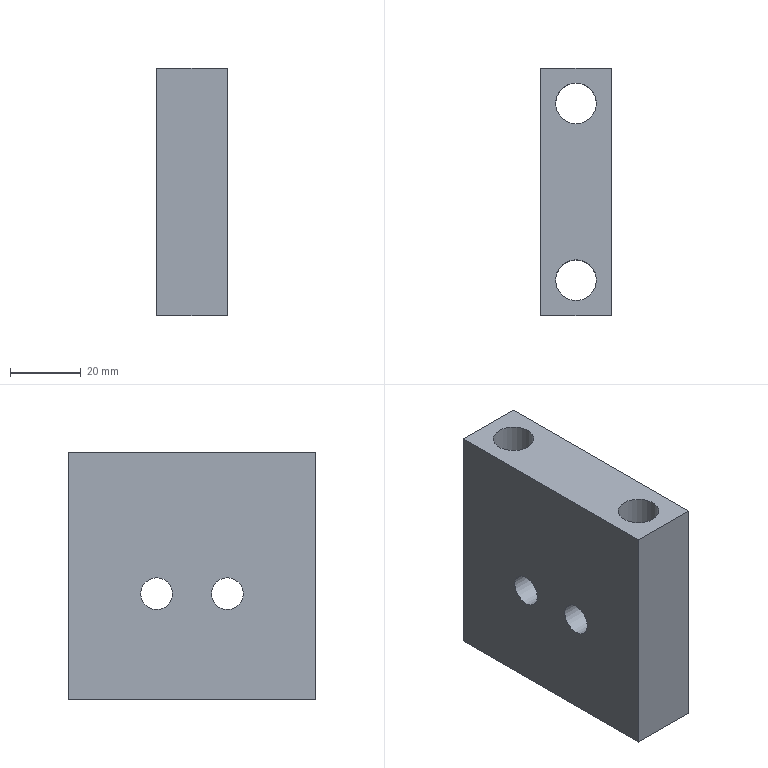Part | NX | features solid 2 | 1 solid | 18 faces | box 20 x 70 x 70 mm | volume 74709 mm3 | plane 10 | cylinder 8 | commonest cylinder face diameters 9 x2 11.5 x2 14 x2 16.5 x2
STEP:
#1=CARTESIAN_POINT('',(-199.,160.,174.5));
#2=VERTEX_POINT('',#1);
#3=CARTESIAN_POINT('',(-199.,160.,170.));
#4=DIRECTION('',(1.,0.,0.));
#5=DIRECTION('',(0.,0.,1.));
#6=AXIS2_PLACEMENT_3D('',#3,#4,#5);
#7=CIRCLE('',#6,4.5);
#8=EDGE_CURVE('',#2,#2,#7,.T.);
#9=ORIENTED_EDGE('',*,*,#8,.T.);
#10=EDGE_LOOP('',(#9));
#11=FACE_BOUND('',#10,.T.);
#12=CARTESIAN_POINT('',(-199.,180.,174.5));
#13=VERTEX_POINT('',#12);
#14=CARTESIAN_POINT('',(-199.,180.,170.));
#15=DIRECTION('',(1.,0.,0.));
#16=DIRECTION('',(0.,0.,1.));
#17=AXIS2_PLACEMENT_3D('',#14,#15,#16);
#18=CIRCLE('',#17,4.5);
#19=EDGE_CURVE('',#13,#13,#18,.T.);
#20=ORIENTED_EDGE('',*,*,#19,.T.);
#21=EDGE_LOOP('',(#20));
#22=FACE_BOUND('',#21,.T.);
#23=CARTESIAN_POINT('',(-199.,205.,210.));
#24=VERTEX_POINT('',#23);
#25=CARTESIAN_POINT('',(-199.,205.,140.));
#26=VERTEX_POINT('',#25);
#27=CARTESIAN_POINT('',(-199.,205.,197.5));
#28=DIRECTION('',(0.,0.,1.));
#29=VECTOR('',#28,1000.);
#30=LINE('',#27,#29);
#31=EDGE_CURVE('',#24,#26,#30,.F.);
#32=ORIENTED_EDGE('',*,*,#31,.T.);
#33=CARTESIAN_POINT('',(-199.,135.,140.));
#34=VERTEX_POINT('',#33);
#35=CARTESIAN_POINT('',(-199.,200.,140.));
#36=DIRECTION('',(0.,-1.,0.));
#37=VECTOR('',#36,1000.);
#38=LINE('',#35,#37);
#39=EDGE_CURVE('',#26,#34,#38,.T.);
#40=ORIENTED_EDGE('',*,*,#39,.T.);
#41=CARTESIAN_POINT('',(-199.,135.,210.));
#42=VERTEX_POINT('',#41);
#43=CARTESIAN_POINT('',(-199.,135.,197.5));
#44=DIRECTION('',(0.,0.,-1.));
#45=VECTOR('',#44,1000.);
#46=LINE('',#43,#45);
#47=EDGE_CURVE('',#42,#34,#46,.T.);
#48=ORIENTED_EDGE('',*,*,#47,.F.);
#49=CARTESIAN_POINT('',(-199.,200.,210.));
#50=DIRECTION('',(0.,-1.,0.));
#51=VECTOR('',#50,1000.);
#52=LINE('',#49,#51);
#53=EDGE_CURVE('',#24,#42,#52,.T.);
#54=ORIENTED_EDGE('',*,*,#53,.F.);
#55=EDGE_LOOP('',(#32,#40,#48,#54));
#56=FACE_BOUND('',#55,.T.);
#57=CARTESIAN_POINT('',(-199.,200.,197.5));
#58=DIRECTION('',(-1.,0.,0.));
#59=DIRECTION('',(0.,-1.,0.));
#60=AXIS2_PLACEMENT_3D('',#57,#58,#59);
#61=PLANE('',#60);
#62=ADVANCED_FACE('',(#11,#22,#56),#61,.T.);
#63=ORIENTED_EDGE('',*,*,#47,.T.);
#64=CARTESIAN_POINT('',(-179.,135.,140.));
#65=VERTEX_POINT('',#64);
#66=CARTESIAN_POINT('',(-199.,135.,140.));
#67=DIRECTION('',(1.,0.,0.));
#68=VECTOR('',#67,1000.);
#69=LINE('',#66,#68);
#70=EDGE_CURVE('',#34,#65,#69,.T.);
#71=ORIENTED_EDGE('',*,*,#70,.T.);
#72=CARTESIAN_POINT('',(-179.,135.,210.));
#73=VERTEX_POINT('',#72);
#74=CARTESIAN_POINT('',(-179.,135.,197.5));
#75=DIRECTION('',(0.,0.,1.));
#76=VECTOR('',#75,1000.);
#77=LINE('',#74,#76);
#78=EDGE_CURVE('',#73,#65,#77,.F.);
#79=ORIENTED_EDGE('',*,*,#78,.F.);
#80=CARTESIAN_POINT('',(-199.,135.,210.));
#81=DIRECTION('',(1.,0.,0.));
#82=VECTOR('',#81,1000.);
#83=LINE('',#80,#82);
#84=EDGE_CURVE('',#42,#73,#83,.T.);
#85=ORIENTED_EDGE('',*,*,#84,.F.);
#86=EDGE_LOOP('',(#63,#71,#79,#85));
#87=FACE_BOUND('',#86,.T.);
#88=CARTESIAN_POINT('',(-199.,135.,197.5));
#89=DIRECTION('',(0.,-1.,0.));
#90=DIRECTION('',(1.,0.,0.));
#91=AXIS2_PLACEMENT_3D('',#88,#89,#90);
#92=PLANE('',#91);
#93=ADVANCED_FACE('',(#87),#92,.T.);
#94=CARTESIAN_POINT('',(-179.,160.,177.));
#95=VERTEX_POINT('',#94);
#96=CARTESIAN_POINT('',(-179.,160.,170.));
#97=DIRECTION('',(1.,0.,0.));
#98=DIRECTION('',(0.,0.,1.));
#99=AXIS2_PLACEMENT_3D('',#96,#97,#98);
#100=CIRCLE('',#99,7.);
#101=EDGE_CURVE('',#95,#95,#100,.T.);
#102=ORIENTED_EDGE('',*,*,#101,.F.);
#103=EDGE_LOOP('',(#102));
#104=FACE_BOUND('',#103,.T.);
#105=CARTESIAN_POINT('',(-179.,180.,177.));
#106=VERTEX_POINT('',#105);
#107=CARTESIAN_POINT('',(-179.,180.,170.));
#108=DIRECTION('',(1.,0.,0.));
#109=DIRECTION('',(0.,0.,1.));
#110=AXIS2_PLACEMENT_3D('',#107,#108,#109);
#111=CIRCLE('',#110,7.);
#112=EDGE_CURVE('',#106,#106,#111,.T.);
#113=ORIENTED_EDGE('',*,*,#112,.F.);
#114=EDGE_LOOP('',(#113));
#115=FACE_BOUND('',#114,.T.);
#116=ORIENTED_EDGE('',*,*,#78,.T.);
#117=CARTESIAN_POINT('',(-179.,205.,140.));
#118=VERTEX_POINT('',#117);
#119=CARTESIAN_POINT('',(-179.,200.,140.));
#120=DIRECTION('',(0.,1.,0.));
#121=VECTOR('',#120,1000.);
#122=LINE('',#119,#121);
#123=EDGE_CURVE('',#118,#65,#122,.F.);
#124=ORIENTED_EDGE('',*,*,#123,.F.);
#125=CARTESIAN_POINT('',(-179.,205.,210.));
#126=VERTEX_POINT('',#125);
#127=CARTESIAN_POINT('',(-179.,205.,197.5));
#128=DIRECTION('',(0.,0.,-1.));
#129=VECTOR('',#128,1000.);
#130=LINE('',#127,#129);
#131=EDGE_CURVE('',#126,#118,#130,.T.);
#132=ORIENTED_EDGE('',*,*,#131,.F.);
#133=CARTESIAN_POINT('',(-179.,200.,210.));
#134=DIRECTION('',(0.,1.,0.));
#135=VECTOR('',#134,1000.);
#136=LINE('',#133,#135);
#137=EDGE_CURVE('',#126,#73,#136,.F.);
#138=ORIENTED_EDGE('',*,*,#137,.T.);
#139=EDGE_LOOP('',(#116,#124,#132,#138));
#140=FACE_BOUND('',#139,.T.);
#141=CARTESIAN_POINT('',(-179.,200.,197.5));
#142=DIRECTION('',(-1.,0.,0.));
#143=DIRECTION('',(0.,-1.,0.));
#144=AXIS2_PLACEMENT_3D('',#141,#142,#143);
#145=PLANE('',#144);
#146=ADVANCED_FACE('',(#104,#115,#140),#145,.F.);
#147=CARTESIAN_POINT('',(-199.,205.,210.));
#148=DIRECTION('',(-1.,0.,0.));
#149=VECTOR('',#148,1000.);
#150=LINE('',#147,#149);
#151=EDGE_CURVE('',#24,#126,#150,.F.);
#152=ORIENTED_EDGE('',*,*,#151,.T.);
#153=ORIENTED_EDGE('',*,*,#131,.T.);
#154=CARTESIAN_POINT('',(-199.,205.,140.));
#155=DIRECTION('',(-1.,0.,0.));
#156=VECTOR('',#155,1000.);
#157=LINE('',#154,#156);
#158=EDGE_CURVE('',#26,#118,#157,.F.);
#159=ORIENTED_EDGE('',*,*,#158,.F.);
#160=ORIENTED_EDGE('',*,*,#31,.F.);
#161=EDGE_LOOP('',(#152,#153,#159,#160));
#162=FACE_BOUND('',#161,.T.);
#163=CARTESIAN_POINT('',(-199.,205.,197.5));
#164=DIRECTION('',(0.,-1.,0.));
#165=DIRECTION('',(1.,0.,0.));
#166=AXIS2_PLACEMENT_3D('',#163,#164,#165);
#167=PLANE('',#166);
#168=ADVANCED_FACE('',(#162),#167,.F.);
#169=CARTESIAN_POINT('',(-189.,186.75,140.));
#170=VERTEX_POINT('',#169);
#171=CARTESIAN_POINT('',(-189.,195.,140.));
#172=DIRECTION('',(0.,0.,-1.));
#173=DIRECTION('',(0.,-1.,0.));
#174=AXIS2_PLACEMENT_3D('',#171,#172,#173);
#175=CIRCLE('',#174,8.25);
#176=EDGE_CURVE('',#170,#170,#175,.T.);
#177=ORIENTED_EDGE('',*,*,#176,.F.);
#178=EDGE_LOOP('',(#177));
#179=FACE_BOUND('',#178,.T.);
#180=CARTESIAN_POINT('',(-189.,136.75,140.));
#181=VERTEX_POINT('',#180);
#182=CARTESIAN_POINT('',(-189.,145.,140.));
#183=DIRECTION('',(0.,0.,-1.));
#184=DIRECTION('',(0.,-1.,0.));
#185=AXIS2_PLACEMENT_3D('',#182,#183,#184);
#186=CIRCLE('',#185,8.25);
#187=EDGE_CURVE('',#181,#181,#186,.T.);
#188=ORIENTED_EDGE('',*,*,#187,.F.);
#189=EDGE_LOOP('',(#188));
#190=FACE_BOUND('',#189,.T.);
#191=ORIENTED_EDGE('',*,*,#123,.T.);
#192=ORIENTED_EDGE('',*,*,#70,.F.);
#193=ORIENTED_EDGE('',*,*,#39,.F.);
#194=ORIENTED_EDGE('',*,*,#158,.T.);
#195=EDGE_LOOP('',(#191,#192,#193,#194));
#196=FACE_BOUND('',#195,.T.);
#197=CARTESIAN_POINT('',(-199.,200.,140.));
#198=DIRECTION('',(0.,0.,-1.));
#199=DIRECTION('',(0.,1.,0.));
#200=AXIS2_PLACEMENT_3D('',#197,#198,#199);
#201=PLANE('',#200);
#202=ADVANCED_FACE('',(#179,#190,#196),#201,.T.);
#203=CARTESIAN_POINT('',(-189.,200.75,210.));
#204=VERTEX_POINT('',#203);
#205=CARTESIAN_POINT('',(-189.,195.,210.));
#206=DIRECTION('',(0.,0.,1.));
#207=DIRECTION('',(0.,1.,0.));
#208=AXIS2_PLACEMENT_3D('',#205,#206,#207);
#209=CIRCLE('',#208,5.75);
#210=EDGE_CURVE('',#204,#204,#209,.T.);
#211=ORIENTED_EDGE('',*,*,#210,.F.);
#212=EDGE_LOOP('',(#211));
#213=FACE_BOUND('',#212,.T.);
#214=CARTESIAN_POINT('',(-189.,150.75,210.));
#215=VERTEX_POINT('',#214);
#216=CARTESIAN_POINT('',(-189.,145.,210.));
#217=DIRECTION('',(0.,0.,1.));
#218=DIRECTION('',(0.,1.,0.));
#219=AXIS2_PLACEMENT_3D('',#216,#217,#218);
#220=CIRCLE('',#219,5.75);
#221=EDGE_CURVE('',#215,#215,#220,.T.);
#222=ORIENTED_EDGE('',*,*,#221,.F.);
#223=EDGE_LOOP('',(#222));
#224=FACE_BOUND('',#223,.T.);
#225=ORIENTED_EDGE('',*,*,#137,.F.);
#226=ORIENTED_EDGE('',*,*,#151,.F.);
#227=ORIENTED_EDGE('',*,*,#53,.T.);
#228=ORIENTED_EDGE('',*,*,#84,.T.);
#229=EDGE_LOOP('',(#225,#226,#227,#228));
#230=FACE_BOUND('',#229,.T.);
#231=CARTESIAN_POINT('',(-199.,200.,210.));
#232=DIRECTION('',(0.,0.,-1.));
#233=DIRECTION('',(0.,1.,0.));
#234=AXIS2_PLACEMENT_3D('',#231,#232,#233);
#235=PLANE('',#234);
#236=ADVANCED_FACE('',(#213,#224,#230),#235,.F.);
#237=ORIENTED_EDGE('',*,*,#19,.F.);
#238=EDGE_LOOP('',(#237));
#239=FACE_BOUND('',#238,.T.);
#240=CARTESIAN_POINT('',(-189.,180.,174.5));
#241=VERTEX_POINT('',#240);
#242=CARTESIAN_POINT('',(-189.,180.,170.));
#243=DIRECTION('',(1.,0.,0.));
#244=DIRECTION('',(0.,0.,1.));
#245=AXIS2_PLACEMENT_3D('',#242,#243,#244);
#246=CIRCLE('',#245,4.5);
#247=EDGE_CURVE('',#241,#241,#246,.T.);
#248=ORIENTED_EDGE('',*,*,#247,.T.);
#249=EDGE_LOOP('',(#248));
#250=FACE_BOUND('',#249,.T.);
#251=CARTESIAN_POINT('',(-229.,180.,170.));
#252=DIRECTION('',(-1.,0.,0.));
#253=DIRECTION('',(0.,0.,1.));
#254=AXIS2_PLACEMENT_3D('',#251,#252,#253);
#255=CYLINDRICAL_SURFACE('',#254,4.5);
#256=ADVANCED_FACE('',(#239,#250),#255,.F.);
#257=ORIENTED_EDGE('',*,*,#247,.F.);
#258=EDGE_LOOP('',(#257));
#259=FACE_BOUND('',#258,.T.);
#260=CARTESIAN_POINT('',(-189.,180.,177.));
#261=VERTEX_POINT('',#260);
#262=CARTESIAN_POINT('',(-189.,180.,170.));
#263=DIRECTION('',(1.,0.,0.));
#264=DIRECTION('',(0.,0.,1.));
#265=AXIS2_PLACEMENT_3D('',#262,#263,#264);
#266=CIRCLE('',#265,7.);
#267=EDGE_CURVE('',#261,#261,#266,.T.);
#268=ORIENTED_EDGE('',*,*,#267,.T.);
#269=EDGE_LOOP('',(#268));
#270=FACE_BOUND('',#269,.T.);
#271=CARTESIAN_POINT('',(-189.,180.,170.));
#272=DIRECTION('',(-1.,0.,0.));
#273=DIRECTION('',(0.,0.,1.));
#274=AXIS2_PLACEMENT_3D('',#271,#272,#273);
#275=PLANE('',#274);
#276=ADVANCED_FACE('',(#259,#270),#275,.F.);
#277=ORIENTED_EDGE('',*,*,#267,.F.);
#278=EDGE_LOOP('',(#277));
#279=FACE_BOUND('',#278,.T.);
#280=ORIENTED_EDGE('',*,*,#112,.T.);
#281=EDGE_LOOP('',(#280));
#282=FACE_BOUND('',#281,.T.);
#283=CARTESIAN_POINT('',(-179.,180.,170.));
#284=DIRECTION('',(-1.,0.,0.));
#285=DIRECTION('',(0.,0.,1.));
#286=AXIS2_PLACEMENT_3D('',#283,#284,#285);
#287=CYLINDRICAL_SURFACE('',#286,7.);
#288=ADVANCED_FACE('',(#279,#282),#287,.F.);
#289=ORIENTED_EDGE('',*,*,#8,.F.);
#290=EDGE_LOOP('',(#289));
#291=FACE_BOUND('',#290,.T.);
#292=CARTESIAN_POINT('',(-189.,160.,174.5));
#293=VERTEX_POINT('',#292);
#294=CARTESIAN_POINT('',(-189.,160.,170.));
#295=DIRECTION('',(1.,0.,0.));
#296=DIRECTION('',(0.,0.,1.));
#297=AXIS2_PLACEMENT_3D('',#294,#295,#296);
#298=CIRCLE('',#297,4.5);
#299=EDGE_CURVE('',#293,#293,#298,.T.);
#300=ORIENTED_EDGE('',*,*,#299,.T.);
#301=EDGE_LOOP('',(#300));
#302=FACE_BOUND('',#301,.T.);
#303=CARTESIAN_POINT('',(-229.,160.,170.));
#304=DIRECTION('',(-1.,0.,0.));
#305=DIRECTION('',(0.,0.,1.));
#306=AXIS2_PLACEMENT_3D('',#303,#304,#305);
#307=CYLINDRICAL_SURFACE('',#306,4.5);
#308=ADVANCED_FACE('',(#291,#302),#307,.F.);
#309=ORIENTED_EDGE('',*,*,#299,.F.);
#310=EDGE_LOOP('',(#309));
#311=FACE_BOUND('',#310,.T.);
#312=CARTESIAN_POINT('',(-189.,160.,177.));
#313=VERTEX_POINT('',#312);
#314=CARTESIAN_POINT('',(-189.,160.,170.));
#315=DIRECTION('',(1.,0.,0.));
#316=DIRECTION('',(0.,0.,1.));
#317=AXIS2_PLACEMENT_3D('',#314,#315,#316);
#318=CIRCLE('',#317,7.);
#319=EDGE_CURVE('',#313,#313,#318,.T.);
#320=ORIENTED_EDGE('',*,*,#319,.T.);
#321=EDGE_LOOP('',(#320));
#322=FACE_BOUND('',#321,.T.);
#323=CARTESIAN_POINT('',(-189.,160.,170.));
#324=DIRECTION('',(-1.,0.,0.));
#325=DIRECTION('',(0.,0.,1.));
#326=AXIS2_PLACEMENT_3D('',#323,#324,#325);
#327=PLANE('',#326);
#328=ADVANCED_FACE('',(#311,#322),#327,.F.);
#329=ORIENTED_EDGE('',*,*,#319,.F.);
#330=EDGE_LOOP('',(#329));
#331=FACE_BOUND('',#330,.T.);
#332=ORIENTED_EDGE('',*,*,#101,.T.);
#333=EDGE_LOOP('',(#332));
#334=FACE_BOUND('',#333,.T.);
#335=CARTESIAN_POINT('',(-179.,160.,170.));
#336=DIRECTION('',(-1.,0.,0.));
#337=DIRECTION('',(0.,0.,1.));
#338=AXIS2_PLACEMENT_3D('',#335,#336,#337);
#339=CYLINDRICAL_SURFACE('',#338,7.);
#340=ADVANCED_FACE('',(#331,#334),#339,.F.);
#341=CARTESIAN_POINT('',(-189.,139.25,160.));
#342=VERTEX_POINT('',#341);
#343=CARTESIAN_POINT('',(-189.,145.,160.));
#344=DIRECTION('',(0.,0.,-1.));
#345=DIRECTION('',(0.,-1.,0.));
#346=AXIS2_PLACEMENT_3D('',#343,#344,#345);
#347=CIRCLE('',#346,5.75);
#348=EDGE_CURVE('',#342,#342,#347,.T.);
#349=ORIENTED_EDGE('',*,*,#348,.T.);
#350=EDGE_LOOP('',(#349));
#351=FACE_BOUND('',#350,.T.);
#352=ORIENTED_EDGE('',*,*,#221,.T.);
#353=EDGE_LOOP('',(#352));
#354=FACE_BOUND('',#353,.T.);
#355=CARTESIAN_POINT('',(-189.,145.,190.));
#356=DIRECTION('',(0.,0.,1.));
#357=DIRECTION('',(0.,-1.,0.));
#358=AXIS2_PLACEMENT_3D('',#355,#356,#357);
#359=CYLINDRICAL_SURFACE('',#358,5.75);
#360=ADVANCED_FACE('',(#351,#354),#359,.F.);
#361=ORIENTED_EDGE('',*,*,#348,.F.);
#362=EDGE_LOOP('',(#361));
#363=FACE_BOUND('',#362,.T.);
#364=CARTESIAN_POINT('',(-189.,136.75,160.));
#365=VERTEX_POINT('',#364);
#366=CARTESIAN_POINT('',(-189.,145.,160.));
#367=DIRECTION('',(0.,0.,-1.));
#368=DIRECTION('',(0.,-1.,0.));
#369=AXIS2_PLACEMENT_3D('',#366,#367,#368);
#370=CIRCLE('',#369,8.25);
#371=EDGE_CURVE('',#365,#365,#370,.T.);
#372=ORIENTED_EDGE('',*,*,#371,.T.);
#373=EDGE_LOOP('',(#372));
#374=FACE_BOUND('',#373,.T.);
#375=CARTESIAN_POINT('',(-189.,145.,160.));
#376=DIRECTION('',(0.,0.,1.));
#377=DIRECTION('',(0.,-1.,0.));
#378=AXIS2_PLACEMENT_3D('',#375,#376,#377);
#379=PLANE('',#378);
#380=ADVANCED_FACE('',(#363,#374),#379,.F.);
#381=ORIENTED_EDGE('',*,*,#371,.F.);
#382=EDGE_LOOP('',(#381));
#383=FACE_BOUND('',#382,.T.);
#384=ORIENTED_EDGE('',*,*,#187,.T.);
#385=EDGE_LOOP('',(#384));
#386=FACE_BOUND('',#385,.T.);
#387=CARTESIAN_POINT('',(-189.,145.,140.));
#388=DIRECTION('',(0.,0.,1.));
#389=DIRECTION('',(0.,-1.,0.));
#390=AXIS2_PLACEMENT_3D('',#387,#388,#389);
#391=CYLINDRICAL_SURFACE('',#390,8.25);
#392=ADVANCED_FACE('',(#383,#386),#391,.F.);
#393=CARTESIAN_POINT('',(-189.,189.25,160.));
#394=VERTEX_POINT('',#393);
#395=CARTESIAN_POINT('',(-189.,195.,160.));
#396=DIRECTION('',(0.,0.,-1.));
#397=DIRECTION('',(0.,-1.,0.));
#398=AXIS2_PLACEMENT_3D('',#395,#396,#397);
#399=CIRCLE('',#398,5.75);
#400=EDGE_CURVE('',#394,#394,#399,.T.);
#401=ORIENTED_EDGE('',*,*,#400,.T.);
#402=EDGE_LOOP('',(#401));
#403=FACE_BOUND('',#402,.T.);
#404=ORIENTED_EDGE('',*,*,#210,.T.);
#405=EDGE_LOOP('',(#404));
#406=FACE_BOUND('',#405,.T.);
#407=CARTESIAN_POINT('',(-189.,195.,190.));
#408=DIRECTION('',(0.,0.,1.));
#409=DIRECTION('',(0.,-1.,0.));
#410=AXIS2_PLACEMENT_3D('',#407,#408,#409);
#411=CYLINDRICAL_SURFACE('',#410,5.75);
#412=ADVANCED_FACE('',(#403,#406),#411,.F.);
#413=ORIENTED_EDGE('',*,*,#400,.F.);
#414=EDGE_LOOP('',(#413));
#415=FACE_BOUND('',#414,.T.);
#416=CARTESIAN_POINT('',(-189.,186.75,160.));
#417=VERTEX_POINT('',#416);
#418=CARTESIAN_POINT('',(-189.,195.,160.));
#419=DIRECTION('',(0.,0.,-1.));
#420=DIRECTION('',(0.,-1.,0.));
#421=AXIS2_PLACEMENT_3D('',#418,#419,#420);
#422=CIRCLE('',#421,8.25);
#423=EDGE_CURVE('',#417,#417,#422,.T.);
#424=ORIENTED_EDGE('',*,*,#423,.T.);
#425=EDGE_LOOP('',(#424));
#426=FACE_BOUND('',#425,.T.);
#427=CARTESIAN_POINT('',(-189.,195.,160.));
#428=DIRECTION('',(0.,0.,1.));
#429=DIRECTION('',(0.,-1.,0.));
#430=AXIS2_PLACEMENT_3D('',#427,#428,#429);
#431=PLANE('',#430);
#432=ADVANCED_FACE('',(#415,#426),#431,.F.);
#433=ORIENTED_EDGE('',*,*,#423,.F.);
#434=EDGE_LOOP('',(#433));
#435=FACE_BOUND('',#434,.T.);
#436=ORIENTED_EDGE('',*,*,#176,.T.);
#437=EDGE_LOOP('',(#436));
#438=FACE_BOUND('',#437,.T.);
#439=CARTESIAN_POINT('',(-189.,195.,140.));
#440=DIRECTION('',(0.,0.,1.));
#441=DIRECTION('',(0.,-1.,0.));
#442=AXIS2_PLACEMENT_3D('',#439,#440,#441);
#443=CYLINDRICAL_SURFACE('',#442,8.25);
#444=ADVANCED_FACE('',(#435,#438),#443,.F.);
#445=CLOSED_SHELL('',(#62,#93,#146,#168,#202,#236,#256,#276,#288,#308,#328,#340,#360,#380,#392,#412,#432,#444));
#446=MANIFOLD_SOLID_BREP('',#445);
#447=(LENGTH_UNIT()NAMED_UNIT(*)SI_UNIT(.MILLI.,.METRE.));
#448=UNCERTAINTY_MEASURE_WITH_UNIT(LENGTH_MEASURE(0.00001),#447,'','');
#449=(NAMED_UNIT(*)PLANE_ANGLE_UNIT()SI_UNIT($,.RADIAN.));
#450=(NAMED_UNIT(*)SI_UNIT($,.STERADIAN.)SOLID_ANGLE_UNIT());
#451=(GEOMETRIC_REPRESENTATION_CONTEXT(3)GLOBAL_UNCERTAINTY_ASSIGNED_CONTEXT((#448))GLOBAL_UNIT_ASSIGNED_CONTEXT((#447,#449,#450))REPRESENTATION_CONTEXT('',''));
#452=ADVANCED_BREP_SHAPE_REPRESENTATION('',(#446),#451);